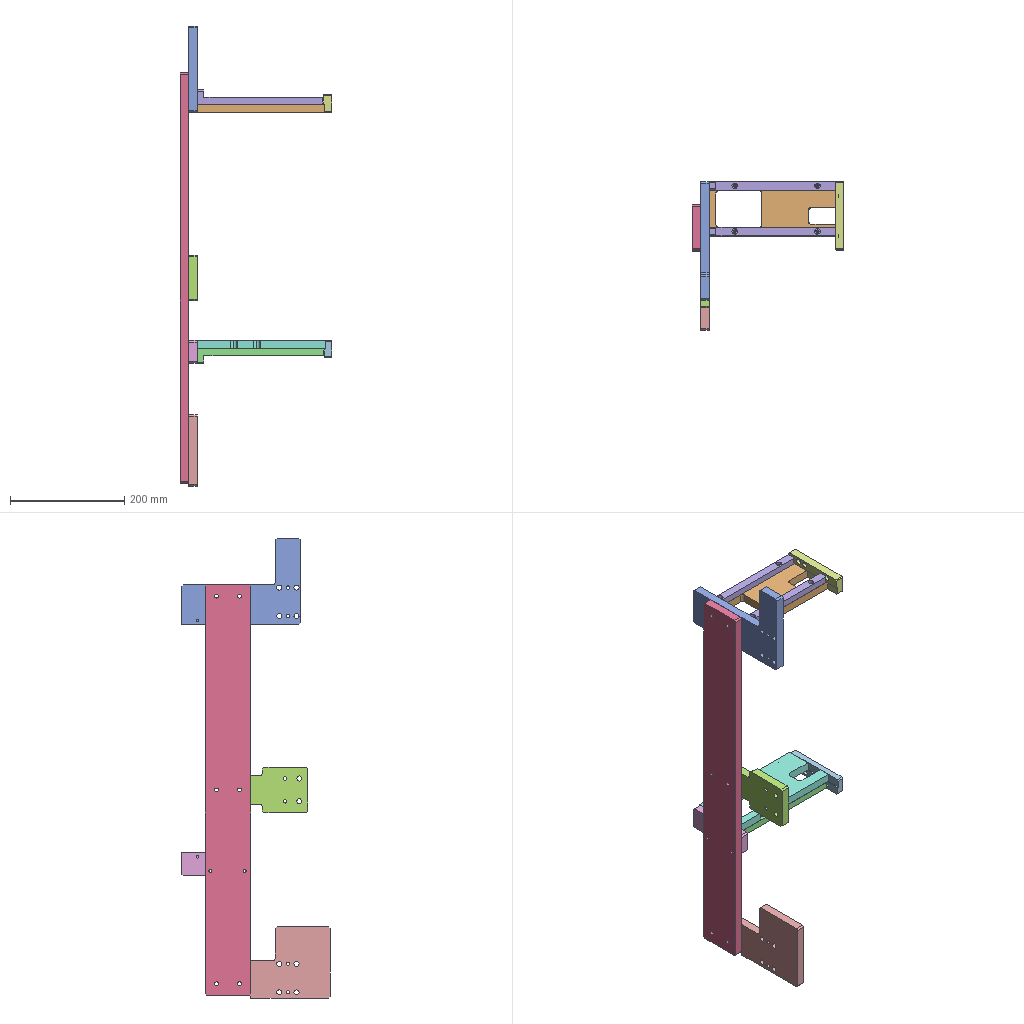Assembly | SolidWorks | 11 different items | 13 placed | box 267 x 260 x 807 mm
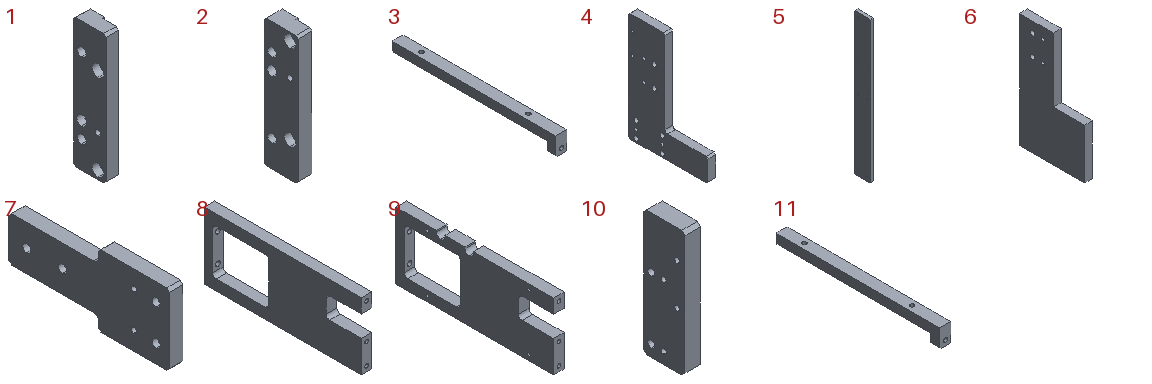Parts list (item | quantity | size | volume | features):
1 | x1 | 13.4 x 30 x 120 mm | 40915 mm3 | features HoleWzd 5, Chamfer 1, Cut 1, Extrusion 1
2 | x1 | 15 x 32 x 120 mm | 49288 mm3 | features HoleWzd 5, Chamfer 1, Cut 1, Extrusion 1
3 | x2 | 15 x 223.1 x 25 mm | 40922 mm3 | features HoleWzd 2, Chamfer 1, Extrusion 1
4 | x1 | 15 x 152.1 x 208 mm | 261148 mm3 | features HoleWzd 9, Chamfer 1, Extrusion 1, Fillet 1, ICE 1
5 | x1 | 15 x 80 x 720 mm | 856123 mm3 | features HoleWzd 7, Chamfer 1, Extrusion 1
6 | x1 | 15 x 125 x 219 mm | 294597 mm3 | features HoleWzd 6, Fillet 2, ICE 2, Chamfer 1, Extrusion 1
7 | x1 | 15 x 180 x 80 mm | 161661 mm3 | features HoleWzd 4, Chamfer 1, Extrusion 1, Fillet 1
8 | x1 | 15 x 223.5 x 95 mm | 215829 mm3 | features HoleWzd 5, Cut 1, Extrusion 1
9 | x1 | 15 x 225.1 x 95 mm | 215693 mm3 | features HoleWzd 5, Cut 2, Extrusion 1, ICE 1, MirrorPattern 1
10 | x1 | 15 x 40 x 121 mm | 68938 mm3 | features HoleWzd 4, Chamfer 1, Extrusion 1
11 | x2 | 15 x 221.5 x 25 mm | 40634 mm3 | features HoleWzd 2, Chamfer 1, Extrusion 1
Mates (type | each side: item.copy, entity, surface, feature):
Coincident | 10.1 face plane Boss-Extrude1 | 9.1 face plane Boss-Extrude1 | 3 times
Coincident | 4.1 face plane Boss-Extrude1 | 10.1 face plane Boss-Extrude1
Coincident | 4.1 face plane Boss-Extrude1 | 8.1 face plane Boss-Extrude1 | 3 times
DistanceDim | 9.1 face plane Boss-Extrude1 | 8.1 face plane Boss-Extrude1
Coincident | 4.1 face plane Boss-Extrude1 | 11.1 face plane Boss-Extrude1 | 2 times
Coincident | 8.1 face plane Boss-Extrude1 | 11.1 face plane Boss-Extrude1
Coincident | 4.1 face plane Boss-Extrude1 | 11.2 face plane Boss-Extrude1
Coincident | 8.1 face plane Boss-Extrude1 | 11.2 face plane Boss-Extrude1 | 2 times
Coincident | 10.1 face plane Boss-Extrude1 | 3.1 face plane Boss-Extrude1
Coincident | 9.1 face plane Boss-Extrude1 | 3.1 face plane Boss-Extrude1 | 2 times
Coincident | 10.1 face plane Boss-Extrude1 | 3.2 face plane Boss-Extrude1
Coincident | 9.1 face plane Cut-Extrude1 | 3.2 face plane Boss-Extrude1 | 2 times
Coincident | 9.1 face plane Boss-Extrude1 | 3.2 face plane Boss-Extrude1
Coincident | 5.1 face plane Boss-Extrude1 | 6.1 face plane Boss-Extrude1 | 2 times
Coincident | 5.1 face plane Boss-Extrude1 | 4.1 face plane Boss-Extrude1 | 2 times
DistanceDim | 5.1 face plane Boss-Extrude1 | 4.1 face plane Boss-Extrude1
Coincident | 5.1 face plane Boss-Extrude1 | 7.1 face plane Boss-Extrude1 | 2 times
Width | 5.1 face plane Boss-Extrude1 | 5.1 face plane Boss-Extrude1 | 7.1 face plane Boss-Extrude1 | 7.1 face plane Boss-Extrude1
Coincident | 5.1 face plane Boss-Extrude1 | 10.1 face plane Boss-Extrude1
Coincident | 8.1 face plane Boss-Extrude1 | 2.1 face plane Cut-Extrude1
Concentric | 8.1 face cylinder M6 Tapped Hole1 | 2.1 face cylinder CBORE for M6 Hexagon socket head cap screws1 | 2 times
Coincident | 9.1 face plane Boss-Extrude1 | 1.1 face plane Cut-Extrude1
Concentric | 1.1 face cylinder CBORE for M6 Hexagon socket head cap screws1 | 9.1 face cylinder M6 Tapped Hole1
Concentric | 9.1 face cylinder Ø5.0mm blind hole 1 | 1.1 face cylinder Ø5.0mm blind hole 1
Concentric | 6.1 face cylinder CBORE for M8 Hexagon socket head cap screws1 | 5.1 face cylinder M8 Tapped Hole1